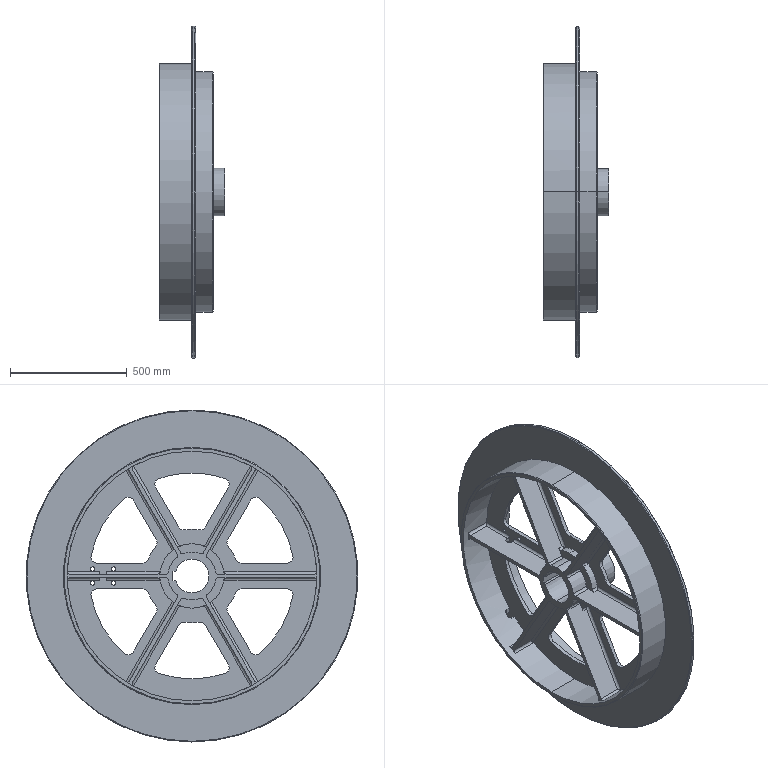Part | SolidWorks | features ICE 5, CirPattern 2, Chamfer 1, Fillet 1, Revolution 1 | 1 solid | 195 faces | box 281 x 1420 x 1420 mm | volume 42495584 mm3 | cylinder 139 | plane 48 | cone 8 | commonest cylinder face diameters 20 x56 50 x28 205 x9 18 x8 275 x7 400 x7